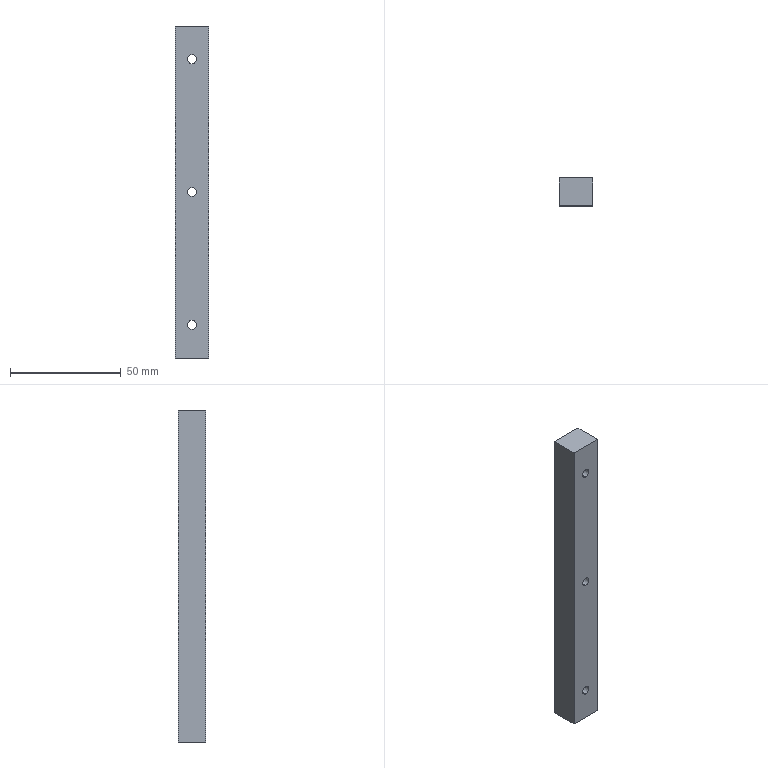Part | SolidWorks | features ICE 3, Extrusion 1, LPattern 1 | 1 solid | 21 faces | box 15 x 12.5 x 150 mm | volume 27442 mm3 | cylinder 12 | plane 9 | commonest cylinder face diameters 4 x6 6 x6
STEP:
#1=CARTESIAN_POINT('',(0.,-6.25,-62.));
#2=VERTEX_POINT('',#1);
#3=CARTESIAN_POINT('',(0.,-6.25,-58.));
#4=VERTEX_POINT('',#3);
#5=CARTESIAN_POINT('',(0.,-6.25,-60.));
#6=DIRECTION('',(0.,1.,0.));
#7=DIRECTION('',(0.,0.,1.));
#8=AXIS2_PLACEMENT_3D('',#5,#6,#7);
#9=CIRCLE('',#8,2.);
#10=EDGE_CURVE('',#2,#4,#9,.T.);
#11=ORIENTED_EDGE('',*,*,#10,.F.);
#12=CARTESIAN_POINT('',(0.,1.75,-62.));
#13=VERTEX_POINT('',#12);
#14=CARTESIAN_POINT('',(0.,-6.25,-62.));
#15=DIRECTION('',(0.,1.,0.));
#16=VECTOR('',#15,1000.);
#17=LINE('',#14,#16);
#18=EDGE_CURVE('',#2,#13,#17,.T.);
#19=ORIENTED_EDGE('',*,*,#18,.T.);
#20=CARTESIAN_POINT('',(0.,1.75,-58.));
#21=VERTEX_POINT('',#20);
#22=CARTESIAN_POINT('',(0.,1.75,-60.));
#23=DIRECTION('',(0.,1.,0.));
#24=DIRECTION('',(0.,0.,1.));
#25=AXIS2_PLACEMENT_3D('',#22,#23,#24);
#26=CIRCLE('',#25,2.);
#27=EDGE_CURVE('',#13,#21,#26,.T.);
#28=ORIENTED_EDGE('',*,*,#27,.T.);
#29=CARTESIAN_POINT('',(0.,-6.25,-58.));
#30=DIRECTION('',(0.,1.,0.));
#31=VECTOR('',#30,1000.);
#32=LINE('',#29,#31);
#33=EDGE_CURVE('',#4,#21,#32,.T.);
#34=ORIENTED_EDGE('',*,*,#33,.F.);
#35=EDGE_LOOP('',(#11,#19,#28,#34));
#36=FACE_OUTER_BOUND('',#35,.T.);
#37=CARTESIAN_POINT('',(0.,-6.25,-60.));
#38=DIRECTION('',(0.,1.,0.));
#39=DIRECTION('',(0.,0.,1.));
#40=AXIS2_PLACEMENT_3D('',#37,#38,#39);
#41=CYLINDRICAL_SURFACE('',#40,2.);
#42=ADVANCED_FACE('',(#36),#41,.F.);
#43=CARTESIAN_POINT('',(0.,-6.25,-2.));
#44=VERTEX_POINT('',#43);
#45=CARTESIAN_POINT('',(0.,-6.25,2.));
#46=VERTEX_POINT('',#45);
#47=CARTESIAN_POINT('',(0.,-6.25,0.));
#48=DIRECTION('',(0.,1.,0.));
#49=DIRECTION('',(0.,0.,1.));
#50=AXIS2_PLACEMENT_3D('',#47,#48,#49);
#51=CIRCLE('',#50,2.);
#52=EDGE_CURVE('',#44,#46,#51,.T.);
#53=ORIENTED_EDGE('',*,*,#52,.F.);
#54=CARTESIAN_POINT('',(0.,1.75,-2.));
#55=VERTEX_POINT('',#54);
#56=CARTESIAN_POINT('',(0.,-6.25,-2.));
#57=DIRECTION('',(0.,1.,0.));
#58=VECTOR('',#57,1000.);
#59=LINE('',#56,#58);
#60=EDGE_CURVE('',#44,#55,#59,.T.);
#61=ORIENTED_EDGE('',*,*,#60,.T.);
#62=CARTESIAN_POINT('',(0.,1.75,2.));
#63=VERTEX_POINT('',#62);
#64=CARTESIAN_POINT('',(0.,1.75,0.));
#65=DIRECTION('',(0.,1.,0.));
#66=DIRECTION('',(0.,0.,1.));
#67=AXIS2_PLACEMENT_3D('',#64,#65,#66);
#68=CIRCLE('',#67,2.);
#69=EDGE_CURVE('',#55,#63,#68,.T.);
#70=ORIENTED_EDGE('',*,*,#69,.T.);
#71=CARTESIAN_POINT('',(0.,-6.25,2.));
#72=DIRECTION('',(0.,1.,0.));
#73=VECTOR('',#72,1000.);
#74=LINE('',#71,#73);
#75=EDGE_CURVE('',#46,#63,#74,.T.);
#76=ORIENTED_EDGE('',*,*,#75,.F.);
#77=EDGE_LOOP('',(#53,#61,#70,#76));
#78=FACE_OUTER_BOUND('',#77,.T.);
#79=CARTESIAN_POINT('',(0.,-6.25,0.));
#80=DIRECTION('',(0.,1.,0.));
#81=DIRECTION('',(0.,0.,1.));
#82=AXIS2_PLACEMENT_3D('',#79,#80,#81);
#83=CYLINDRICAL_SURFACE('',#82,2.);
#84=ADVANCED_FACE('',(#78),#83,.F.);
#85=CARTESIAN_POINT('',(0.,1.75,-63.));
#86=VERTEX_POINT('',#85);
#87=CARTESIAN_POINT('',(0.,1.75,-57.));
#88=VERTEX_POINT('',#87);
#89=CARTESIAN_POINT('',(0.,1.75,-60.));
#90=DIRECTION('',(0.,1.,0.));
#91=DIRECTION('',(0.,0.,1.));
#92=AXIS2_PLACEMENT_3D('',#89,#90,#91);
#93=CIRCLE('',#92,3.);
#94=EDGE_CURVE('',#86,#88,#93,.T.);
#95=ORIENTED_EDGE('',*,*,#94,.F.);
#96=CARTESIAN_POINT('',(0.,6.25,-63.));
#97=VERTEX_POINT('',#96);
#98=CARTESIAN_POINT('',(0.,1.75,-63.));
#99=DIRECTION('',(0.,1.,0.));
#100=VECTOR('',#99,1000.);
#101=LINE('',#98,#100);
#102=EDGE_CURVE('',#86,#97,#101,.T.);
#103=ORIENTED_EDGE('',*,*,#102,.T.);
#104=CARTESIAN_POINT('',(0.,6.25,-57.));
#105=VERTEX_POINT('',#104);
#106=CARTESIAN_POINT('',(0.,6.25,-60.));
#107=DIRECTION('',(0.,1.,0.));
#108=DIRECTION('',(0.,0.,1.));
#109=AXIS2_PLACEMENT_3D('',#106,#107,#108);
#110=CIRCLE('',#109,3.);
#111=EDGE_CURVE('',#97,#105,#110,.T.);
#112=ORIENTED_EDGE('',*,*,#111,.T.);
#113=CARTESIAN_POINT('',(0.,1.75,-57.));
#114=DIRECTION('',(0.,1.,0.));
#115=VECTOR('',#114,1000.);
#116=LINE('',#113,#115);
#117=EDGE_CURVE('',#88,#105,#116,.T.);
#118=ORIENTED_EDGE('',*,*,#117,.F.);
#119=EDGE_LOOP('',(#95,#103,#112,#118));
#120=FACE_OUTER_BOUND('',#119,.T.);
#121=CARTESIAN_POINT('',(0.,1.75,-60.));
#122=DIRECTION('',(0.,1.,0.));
#123=DIRECTION('',(0.,0.,1.));
#124=AXIS2_PLACEMENT_3D('',#121,#122,#123);
#125=CYLINDRICAL_SURFACE('',#124,3.);
#126=ADVANCED_FACE('',(#120),#125,.F.);
#127=CARTESIAN_POINT('',(0.,1.75,-3.));
#128=VERTEX_POINT('',#127);
#129=CARTESIAN_POINT('',(0.,1.75,3.));
#130=VERTEX_POINT('',#129);
#131=CARTESIAN_POINT('',(0.,1.75,0.));
#132=DIRECTION('',(0.,1.,0.));
#133=DIRECTION('',(0.,0.,1.));
#134=AXIS2_PLACEMENT_3D('',#131,#132,#133);
#135=CIRCLE('',#134,3.);
#136=EDGE_CURVE('',#128,#130,#135,.T.);
#137=ORIENTED_EDGE('',*,*,#136,.F.);
#138=CARTESIAN_POINT('',(0.,6.25,-3.));
#139=VERTEX_POINT('',#138);
#140=CARTESIAN_POINT('',(0.,1.75,-3.));
#141=DIRECTION('',(0.,1.,0.));
#142=VECTOR('',#141,1000.);
#143=LINE('',#140,#142);
#144=EDGE_CURVE('',#128,#139,#143,.T.);
#145=ORIENTED_EDGE('',*,*,#144,.T.);
#146=CARTESIAN_POINT('',(0.,6.25,3.));
#147=VERTEX_POINT('',#146);
#148=CARTESIAN_POINT('',(0.,6.25,0.));
#149=DIRECTION('',(0.,1.,0.));
#150=DIRECTION('',(0.,0.,1.));
#151=AXIS2_PLACEMENT_3D('',#148,#149,#150);
#152=CIRCLE('',#151,3.);
#153=EDGE_CURVE('',#139,#147,#152,.T.);
#154=ORIENTED_EDGE('',*,*,#153,.T.);
#155=CARTESIAN_POINT('',(0.,1.75,3.));
#156=DIRECTION('',(0.,1.,0.));
#157=VECTOR('',#156,1000.);
#158=LINE('',#155,#157);
#159=EDGE_CURVE('',#130,#147,#158,.T.);
#160=ORIENTED_EDGE('',*,*,#159,.F.);
#161=EDGE_LOOP('',(#137,#145,#154,#160));
#162=FACE_OUTER_BOUND('',#161,.T.);
#163=CARTESIAN_POINT('',(0.,1.75,0.));
#164=DIRECTION('',(0.,1.,0.));
#165=DIRECTION('',(0.,0.,1.));
#166=AXIS2_PLACEMENT_3D('',#163,#164,#165);
#167=CYLINDRICAL_SURFACE('',#166,3.);
#168=ADVANCED_FACE('',(#162),#167,.F.);
#169=CARTESIAN_POINT('',(0.,-6.25,58.));
#170=VERTEX_POINT('',#169);
#171=CARTESIAN_POINT('',(0.,-6.25,62.));
#172=VERTEX_POINT('',#171);
#173=CARTESIAN_POINT('',(0.,-6.25,60.));
#174=DIRECTION('',(0.,1.,0.));
#175=DIRECTION('',(0.,0.,1.));
#176=AXIS2_PLACEMENT_3D('',#173,#174,#175);
#177=CIRCLE('',#176,2.);
#178=EDGE_CURVE('',#170,#172,#177,.T.);
#179=ORIENTED_EDGE('',*,*,#178,.F.);
#180=CARTESIAN_POINT('',(0.,1.75,58.));
#181=VERTEX_POINT('',#180);
#182=CARTESIAN_POINT('',(0.,-6.25,58.));
#183=DIRECTION('',(0.,1.,0.));
#184=VECTOR('',#183,1000.);
#185=LINE('',#182,#184);
#186=EDGE_CURVE('',#170,#181,#185,.T.);
#187=ORIENTED_EDGE('',*,*,#186,.T.);
#188=CARTESIAN_POINT('',(0.,1.75,62.));
#189=VERTEX_POINT('',#188);
#190=CARTESIAN_POINT('',(0.,1.75,60.));
#191=DIRECTION('',(0.,1.,0.));
#192=DIRECTION('',(0.,0.,1.));
#193=AXIS2_PLACEMENT_3D('',#190,#191,#192);
#194=CIRCLE('',#193,2.);
#195=EDGE_CURVE('',#181,#189,#194,.T.);
#196=ORIENTED_EDGE('',*,*,#195,.T.);
#197=CARTESIAN_POINT('',(0.,-6.25,62.));
#198=DIRECTION('',(0.,1.,0.));
#199=VECTOR('',#198,1000.);
#200=LINE('',#197,#199);
#201=EDGE_CURVE('',#172,#189,#200,.T.);
#202=ORIENTED_EDGE('',*,*,#201,.F.);
#203=EDGE_LOOP('',(#179,#187,#196,#202));
#204=FACE_OUTER_BOUND('',#203,.T.);
#205=CARTESIAN_POINT('',(0.,-6.25,60.));
#206=DIRECTION('',(0.,1.,0.));
#207=DIRECTION('',(0.,0.,1.));
#208=AXIS2_PLACEMENT_3D('',#205,#206,#207);
#209=CYLINDRICAL_SURFACE('',#208,2.);
#210=ADVANCED_FACE('',(#204),#209,.F.);
#211=CARTESIAN_POINT('',(0.,1.75,57.));
#212=VERTEX_POINT('',#211);
#213=CARTESIAN_POINT('',(0.,1.75,63.));
#214=VERTEX_POINT('',#213);
#215=CARTESIAN_POINT('',(0.,1.75,60.));
#216=DIRECTION('',(0.,1.,0.));
#217=DIRECTION('',(0.,0.,1.));
#218=AXIS2_PLACEMENT_3D('',#215,#216,#217);
#219=CIRCLE('',#218,3.);
#220=EDGE_CURVE('',#212,#214,#219,.T.);
#221=ORIENTED_EDGE('',*,*,#220,.F.);
#222=CARTESIAN_POINT('',(0.,6.25,57.));
#223=VERTEX_POINT('',#222);
#224=CARTESIAN_POINT('',(0.,1.75,57.));
#225=DIRECTION('',(0.,1.,0.));
#226=VECTOR('',#225,1000.);
#227=LINE('',#224,#226);
#228=EDGE_CURVE('',#212,#223,#227,.T.);
#229=ORIENTED_EDGE('',*,*,#228,.T.);
#230=CARTESIAN_POINT('',(0.,6.25,63.));
#231=VERTEX_POINT('',#230);
#232=CARTESIAN_POINT('',(0.,6.25,60.));
#233=DIRECTION('',(0.,1.,0.));
#234=DIRECTION('',(0.,0.,1.));
#235=AXIS2_PLACEMENT_3D('',#232,#233,#234);
#236=CIRCLE('',#235,3.);
#237=EDGE_CURVE('',#223,#231,#236,.T.);
#238=ORIENTED_EDGE('',*,*,#237,.T.);
#239=CARTESIAN_POINT('',(0.,1.75,63.));
#240=DIRECTION('',(0.,1.,0.));
#241=VECTOR('',#240,1000.);
#242=LINE('',#239,#241);
#243=EDGE_CURVE('',#214,#231,#242,.T.);
#244=ORIENTED_EDGE('',*,*,#243,.F.);
#245=EDGE_LOOP('',(#221,#229,#238,#244));
#246=FACE_OUTER_BOUND('',#245,.T.);
#247=CARTESIAN_POINT('',(0.,1.75,60.));
#248=DIRECTION('',(0.,1.,0.));
#249=DIRECTION('',(0.,0.,1.));
#250=AXIS2_PLACEMENT_3D('',#247,#248,#249);
#251=CYLINDRICAL_SURFACE('',#250,3.);
#252=ADVANCED_FACE('',(#246),#251,.F.);
#253=CARTESIAN_POINT('',(7.5,-6.25,-75.));
#254=VERTEX_POINT('',#253);
#255=CARTESIAN_POINT('',(7.5,6.25,-75.));
#256=VERTEX_POINT('',#255);
#257=CARTESIAN_POINT('',(7.5,6.25,-75.));
#258=DIRECTION('',(0.,1.,0.));
#259=VECTOR('',#258,1000.);
#260=LINE('',#257,#259);
#261=EDGE_CURVE('',#254,#256,#260,.T.);
#262=ORIENTED_EDGE('',*,*,#261,.T.);
#263=CARTESIAN_POINT('',(7.5,6.25,75.));
#264=VERTEX_POINT('',#263);
#265=CARTESIAN_POINT('',(7.5,6.25,75.));
#266=DIRECTION('',(0.,0.,-1.));
#267=VECTOR('',#266,1000.);
#268=LINE('',#265,#267);
#269=EDGE_CURVE('',#264,#256,#268,.T.);
#270=ORIENTED_EDGE('',*,*,#269,.F.);
#271=CARTESIAN_POINT('',(7.5,-6.25,75.));
#272=VERTEX_POINT('',#271);
#273=CARTESIAN_POINT('',(7.5,6.25,75.));
#274=DIRECTION('',(0.,1.,0.));
#275=VECTOR('',#274,1000.);
#276=LINE('',#273,#275);
#277=EDGE_CURVE('',#272,#264,#276,.T.);
#278=ORIENTED_EDGE('',*,*,#277,.F.);
#279=CARTESIAN_POINT('',(7.5,-6.25,75.));
#280=DIRECTION('',(0.,0.,-1.));
#281=VECTOR('',#280,1000.);
#282=LINE('',#279,#281);
#283=EDGE_CURVE('',#272,#254,#282,.T.);
#284=ORIENTED_EDGE('',*,*,#283,.T.);
#285=EDGE_LOOP('',(#262,#270,#278,#284));
#286=FACE_OUTER_BOUND('',#285,.T.);
#287=CARTESIAN_POINT('',(7.5,6.25,75.));
#288=DIRECTION('',(-1.,0.,0.));
#289=DIRECTION('',(0.,-1.,0.));
#290=AXIS2_PLACEMENT_3D('',#287,#288,#289);
#291=PLANE('',#290);
#292=ADVANCED_FACE('',(#286),#291,.F.);
#293=CARTESIAN_POINT('',(0.,6.25,-60.));
#294=DIRECTION('',(0.,1.,0.));
#295=DIRECTION('',(0.,0.,1.));
#296=AXIS2_PLACEMENT_3D('',#293,#294,#295);
#297=CIRCLE('',#296,3.);
#298=EDGE_CURVE('',#105,#97,#297,.T.);
#299=ORIENTED_EDGE('',*,*,#298,.F.);
#300=ORIENTED_EDGE('',*,*,#111,.F.);
#301=EDGE_LOOP('',(#299,#300));
#302=FACE_BOUND('',#301,.T.);
#303=CARTESIAN_POINT('',(0.,6.25,0.));
#304=DIRECTION('',(0.,1.,0.));
#305=DIRECTION('',(0.,0.,1.));
#306=AXIS2_PLACEMENT_3D('',#303,#304,#305);
#307=CIRCLE('',#306,3.);
#308=EDGE_CURVE('',#147,#139,#307,.T.);
#309=ORIENTED_EDGE('',*,*,#308,.F.);
#310=ORIENTED_EDGE('',*,*,#153,.F.);
#311=EDGE_LOOP('',(#309,#310));
#312=FACE_BOUND('',#311,.T.);
#313=CARTESIAN_POINT('',(0.,6.25,60.));
#314=DIRECTION('',(0.,1.,0.));
#315=DIRECTION('',(0.,0.,1.));
#316=AXIS2_PLACEMENT_3D('',#313,#314,#315);
#317=CIRCLE('',#316,3.);
#318=EDGE_CURVE('',#231,#223,#317,.T.);
#319=ORIENTED_EDGE('',*,*,#318,.F.);
#320=ORIENTED_EDGE('',*,*,#237,.F.);
#321=EDGE_LOOP('',(#319,#320));
#322=FACE_BOUND('',#321,.T.);
#323=CARTESIAN_POINT('',(-7.5,6.25,-75.));
#324=VERTEX_POINT('',#323);
#325=CARTESIAN_POINT('',(-7.5,6.25,-75.));
#326=DIRECTION('',(-1.,0.,0.));
#327=VECTOR('',#326,1000.);
#328=LINE('',#325,#327);
#329=EDGE_CURVE('',#256,#324,#328,.T.);
#330=ORIENTED_EDGE('',*,*,#329,.T.);
#331=CARTESIAN_POINT('',(-7.5,6.25,75.));
#332=VERTEX_POINT('',#331);
#333=CARTESIAN_POINT('',(-7.5,6.25,75.));
#334=DIRECTION('',(0.,0.,-1.));
#335=VECTOR('',#334,1000.);
#336=LINE('',#333,#335);
#337=EDGE_CURVE('',#332,#324,#336,.T.);
#338=ORIENTED_EDGE('',*,*,#337,.F.);
#339=CARTESIAN_POINT('',(-7.5,6.25,75.));
#340=DIRECTION('',(-1.,0.,0.));
#341=VECTOR('',#340,1000.);
#342=LINE('',#339,#341);
#343=EDGE_CURVE('',#264,#332,#342,.T.);
#344=ORIENTED_EDGE('',*,*,#343,.F.);
#345=ORIENTED_EDGE('',*,*,#269,.T.);
#346=EDGE_LOOP('',(#330,#338,#344,#345));
#347=FACE_OUTER_BOUND('',#346,.T.);
#348=CARTESIAN_POINT('',(-7.5,6.25,75.));
#349=DIRECTION('',(0.,-1.,0.));
#350=DIRECTION('',(0.,0.,-1.));
#351=AXIS2_PLACEMENT_3D('',#348,#349,#350);
#352=PLANE('',#351);
#353=ADVANCED_FACE('',(#302,#312,#322,#347),#352,.F.);
#354=CARTESIAN_POINT('',(-7.5,-6.25,-75.));
#355=VERTEX_POINT('',#354);
#356=CARTESIAN_POINT('',(-7.5,6.25,-75.));
#357=DIRECTION('',(0.,-1.,0.));
#358=VECTOR('',#357,1000.);
#359=LINE('',#356,#358);
#360=EDGE_CURVE('',#324,#355,#359,.T.);
#361=ORIENTED_EDGE('',*,*,#360,.T.);
#362=CARTESIAN_POINT('',(-7.5,-6.25,75.));
#363=VERTEX_POINT('',#362);
#364=CARTESIAN_POINT('',(-7.5,-6.25,75.));
#365=DIRECTION('',(0.,0.,-1.));
#366=VECTOR('',#365,1000.);
#367=LINE('',#364,#366);
#368=EDGE_CURVE('',#363,#355,#367,.T.);
#369=ORIENTED_EDGE('',*,*,#368,.F.);
#370=CARTESIAN_POINT('',(-7.5,6.25,75.));
#371=DIRECTION('',(0.,-1.,0.));
#372=VECTOR('',#371,1000.);
#373=LINE('',#370,#372);
#374=EDGE_CURVE('',#332,#363,#373,.T.);
#375=ORIENTED_EDGE('',*,*,#374,.F.);
#376=ORIENTED_EDGE('',*,*,#337,.T.);
#377=EDGE_LOOP('',(#361,#369,#375,#376));
#378=FACE_OUTER_BOUND('',#377,.T.);
#379=CARTESIAN_POINT('',(-7.5,6.25,75.));
#380=DIRECTION('',(1.,0.,0.));
#381=DIRECTION('',(0.,1.,0.));
#382=AXIS2_PLACEMENT_3D('',#379,#380,#381);
#383=PLANE('',#382);
#384=ADVANCED_FACE('',(#378),#383,.F.);
#385=CARTESIAN_POINT('',(0.,-6.25,-60.));
#386=DIRECTION('',(0.,1.,0.));
#387=DIRECTION('',(0.,0.,1.));
#388=AXIS2_PLACEMENT_3D('',#385,#386,#387);
#389=CIRCLE('',#388,2.);
#390=EDGE_CURVE('',#4,#2,#389,.T.);
#391=ORIENTED_EDGE('',*,*,#390,.T.);
#392=ORIENTED_EDGE('',*,*,#10,.T.);
#393=EDGE_LOOP('',(#391,#392));
#394=FACE_BOUND('',#393,.T.);
#395=CARTESIAN_POINT('',(0.,-6.25,0.));
#396=DIRECTION('',(0.,1.,0.));
#397=DIRECTION('',(0.,0.,1.));
#398=AXIS2_PLACEMENT_3D('',#395,#396,#397);
#399=CIRCLE('',#398,2.);
#400=EDGE_CURVE('',#46,#44,#399,.T.);
#401=ORIENTED_EDGE('',*,*,#400,.T.);
#402=ORIENTED_EDGE('',*,*,#52,.T.);
#403=EDGE_LOOP('',(#401,#402));
#404=FACE_BOUND('',#403,.T.);
#405=CARTESIAN_POINT('',(0.,-6.25,60.));
#406=DIRECTION('',(0.,1.,0.));
#407=DIRECTION('',(0.,0.,1.));
#408=AXIS2_PLACEMENT_3D('',#405,#406,#407);
#409=CIRCLE('',#408,2.);
#410=EDGE_CURVE('',#172,#170,#409,.T.);
#411=ORIENTED_EDGE('',*,*,#410,.T.);
#412=ORIENTED_EDGE('',*,*,#178,.T.);
#413=EDGE_LOOP('',(#411,#412));
#414=FACE_BOUND('',#413,.T.);
#415=CARTESIAN_POINT('',(-7.5,-6.25,-75.));
#416=DIRECTION('',(1.,0.,0.));
#417=VECTOR('',#416,1000.);
#418=LINE('',#415,#417);
#419=EDGE_CURVE('',#355,#254,#418,.T.);
#420=ORIENTED_EDGE('',*,*,#419,.T.);
#421=ORIENTED_EDGE('',*,*,#283,.F.);
#422=CARTESIAN_POINT('',(-7.5,-6.25,75.));
#423=DIRECTION('',(1.,0.,0.));
#424=VECTOR('',#423,1000.);
#425=LINE('',#422,#424);
#426=EDGE_CURVE('',#363,#272,#425,.T.);
#427=ORIENTED_EDGE('',*,*,#426,.F.);
#428=ORIENTED_EDGE('',*,*,#368,.T.);
#429=EDGE_LOOP('',(#420,#421,#427,#428));
#430=FACE_OUTER_BOUND('',#429,.T.);
#431=CARTESIAN_POINT('',(-7.5,-6.25,75.));
#432=DIRECTION('',(0.,1.,0.));
#433=DIRECTION('',(0.,0.,1.));
#434=AXIS2_PLACEMENT_3D('',#431,#432,#433);
#435=PLANE('',#434);
#436=ADVANCED_FACE('',(#394,#404,#414,#430),#435,.F.);
#437=ORIENTED_EDGE('',*,*,#277,.T.);
#438=ORIENTED_EDGE('',*,*,#343,.T.);
#439=ORIENTED_EDGE('',*,*,#374,.T.);
#440=ORIENTED_EDGE('',*,*,#426,.T.);
#441=EDGE_LOOP('',(#437,#438,#439,#440));
#442=FACE_OUTER_BOUND('',#441,.T.);
#443=CARTESIAN_POINT('',(0.,0.,75.));
#444=DIRECTION('',(0.,0.,1.));
#445=DIRECTION('',(1.,0.,0.));
#446=AXIS2_PLACEMENT_3D('',#443,#444,#445);
#447=PLANE('',#446);
#448=ADVANCED_FACE('',(#442),#447,.T.);
#449=ORIENTED_EDGE('',*,*,#261,.F.);
#450=ORIENTED_EDGE('',*,*,#419,.F.);
#451=ORIENTED_EDGE('',*,*,#360,.F.);
#452=ORIENTED_EDGE('',*,*,#329,.F.);
#453=EDGE_LOOP('',(#449,#450,#451,#452));
#454=FACE_OUTER_BOUND('',#453,.T.);
#455=CARTESIAN_POINT('',(0.,0.,-75.));
#456=DIRECTION('',(0.,0.,1.));
#457=DIRECTION('',(1.,0.,0.));
#458=AXIS2_PLACEMENT_3D('',#455,#456,#457);
#459=PLANE('',#458);
#460=ADVANCED_FACE('',(#454),#459,.F.);
#461=ORIENTED_EDGE('',*,*,#228,.F.);
#462=CARTESIAN_POINT('',(0.,1.75,60.));
#463=DIRECTION('',(0.,1.,0.));
#464=DIRECTION('',(0.,0.,1.));
#465=AXIS2_PLACEMENT_3D('',#462,#463,#464);
#466=CIRCLE('',#465,3.);
#467=EDGE_CURVE('',#214,#212,#466,.T.);
#468=ORIENTED_EDGE('',*,*,#467,.F.);
#469=ORIENTED_EDGE('',*,*,#243,.T.);
#470=ORIENTED_EDGE('',*,*,#318,.T.);
#471=EDGE_LOOP('',(#461,#468,#469,#470));
#472=FACE_OUTER_BOUND('',#471,.T.);
#473=CARTESIAN_POINT('',(0.,1.75,60.));
#474=DIRECTION('',(0.,1.,0.));
#475=DIRECTION('',(0.,0.,1.));
#476=AXIS2_PLACEMENT_3D('',#473,#474,#475);
#477=CYLINDRICAL_SURFACE('',#476,3.);
#478=ADVANCED_FACE('',(#472),#477,.F.);
#479=CARTESIAN_POINT('',(0.,1.75,60.));
#480=DIRECTION('',(0.,1.,0.));
#481=DIRECTION('',(0.,0.,1.));
#482=AXIS2_PLACEMENT_3D('',#479,#480,#481);
#483=CIRCLE('',#482,2.);
#484=EDGE_CURVE('',#189,#181,#483,.T.);
#485=ORIENTED_EDGE('',*,*,#484,.F.);
#486=ORIENTED_EDGE('',*,*,#195,.F.);
#487=EDGE_LOOP('',(#485,#486));
#488=FACE_BOUND('',#487,.T.);
#489=ORIENTED_EDGE('',*,*,#467,.T.);
#490=ORIENTED_EDGE('',*,*,#220,.T.);
#491=EDGE_LOOP('',(#489,#490));
#492=FACE_OUTER_BOUND('',#491,.T.);
#493=CARTESIAN_POINT('',(0.,1.75,60.));
#494=DIRECTION('',(0.,1.,0.));
#495=DIRECTION('',(0.,0.,1.));
#496=AXIS2_PLACEMENT_3D('',#493,#494,#495);
#497=PLANE('',#496);
#498=ADVANCED_FACE('',(#488,#492),#497,.T.);
#499=ORIENTED_EDGE('',*,*,#186,.F.);
#500=ORIENTED_EDGE('',*,*,#410,.F.);
#501=ORIENTED_EDGE('',*,*,#201,.T.);
#502=ORIENTED_EDGE('',*,*,#484,.T.);
#503=EDGE_LOOP('',(#499,#500,#501,#502));
#504=FACE_OUTER_BOUND('',#503,.T.);
#505=CARTESIAN_POINT('',(0.,-6.25,60.));
#506=DIRECTION('',(0.,1.,0.));
#507=DIRECTION('',(0.,0.,1.));
#508=AXIS2_PLACEMENT_3D('',#505,#506,#507);
#509=CYLINDRICAL_SURFACE('',#508,2.);
#510=ADVANCED_FACE('',(#504),#509,.F.);
#511=ORIENTED_EDGE('',*,*,#144,.F.);
#512=CARTESIAN_POINT('',(0.,1.75,0.));
#513=DIRECTION('',(0.,1.,0.));
#514=DIRECTION('',(0.,0.,1.));
#515=AXIS2_PLACEMENT_3D('',#512,#513,#514);
#516=CIRCLE('',#515,3.);
#517=EDGE_CURVE('',#130,#128,#516,.T.);
#518=ORIENTED_EDGE('',*,*,#517,.F.);
#519=ORIENTED_EDGE('',*,*,#159,.T.);
#520=ORIENTED_EDGE('',*,*,#308,.T.);
#521=EDGE_LOOP('',(#511,#518,#519,#520));
#522=FACE_OUTER_BOUND('',#521,.T.);
#523=CARTESIAN_POINT('',(0.,1.75,0.));
#524=DIRECTION('',(0.,1.,0.));
#525=DIRECTION('',(0.,0.,1.));
#526=AXIS2_PLACEMENT_3D('',#523,#524,#525);
#527=CYLINDRICAL_SURFACE('',#526,3.);
#528=ADVANCED_FACE('',(#522),#527,.F.);
#529=CARTESIAN_POINT('',(0.,1.75,0.));
#530=DIRECTION('',(0.,1.,0.));
#531=DIRECTION('',(0.,0.,1.));
#532=AXIS2_PLACEMENT_3D('',#529,#530,#531);
#533=CIRCLE('',#532,2.);
#534=EDGE_CURVE('',#63,#55,#533,.T.);
#535=ORIENTED_EDGE('',*,*,#534,.F.);
#536=ORIENTED_EDGE('',*,*,#69,.F.);
#537=EDGE_LOOP('',(#535,#536));
#538=FACE_BOUND('',#537,.T.);
#539=ORIENTED_EDGE('',*,*,#517,.T.);
#540=ORIENTED_EDGE('',*,*,#136,.T.);
#541=EDGE_LOOP('',(#539,#540));
#542=FACE_OUTER_BOUND('',#541,.T.);
#543=CARTESIAN_POINT('',(0.,1.75,0.));
#544=DIRECTION('',(0.,1.,0.));
#545=DIRECTION('',(0.,0.,1.));
#546=AXIS2_PLACEMENT_3D('',#543,#544,#545);
#547=PLANE('',#546);
#548=ADVANCED_FACE('',(#538,#542),#547,.T.);
#549=ORIENTED_EDGE('',*,*,#102,.F.);
#550=CARTESIAN_POINT('',(0.,1.75,-60.));
#551=DIRECTION('',(0.,1.,0.));
#552=DIRECTION('',(0.,0.,1.));
#553=AXIS2_PLACEMENT_3D('',#550,#551,#552);
#554=CIRCLE('',#553,3.);
#555=EDGE_CURVE('',#88,#86,#554,.T.);
#556=ORIENTED_EDGE('',*,*,#555,.F.);
#557=ORIENTED_EDGE('',*,*,#117,.T.);
#558=ORIENTED_EDGE('',*,*,#298,.T.);
#559=EDGE_LOOP('',(#549,#556,#557,#558));
#560=FACE_OUTER_BOUND('',#559,.T.);
#561=CARTESIAN_POINT('',(0.,1.75,-60.));
#562=DIRECTION('',(0.,1.,0.));
#563=DIRECTION('',(0.,0.,1.));
#564=AXIS2_PLACEMENT_3D('',#561,#562,#563);
#565=CYLINDRICAL_SURFACE('',#564,3.);
#566=ADVANCED_FACE('',(#560),#565,.F.);
#567=CARTESIAN_POINT('',(0.,1.75,-60.));
#568=DIRECTION('',(0.,1.,0.));
#569=DIRECTION('',(0.,0.,1.));
#570=AXIS2_PLACEMENT_3D('',#567,#568,#569);
#571=CIRCLE('',#570,2.);
#572=EDGE_CURVE('',#21,#13,#571,.T.);
#573=ORIENTED_EDGE('',*,*,#572,.F.);
#574=ORIENTED_EDGE('',*,*,#27,.F.);
#575=EDGE_LOOP('',(#573,#574));
#576=FACE_BOUND('',#575,.T.);
#577=ORIENTED_EDGE('',*,*,#555,.T.);
#578=ORIENTED_EDGE('',*,*,#94,.T.);
#579=EDGE_LOOP('',(#577,#578));
#580=FACE_OUTER_BOUND('',#579,.T.);
#581=CARTESIAN_POINT('',(0.,1.75,-60.));
#582=DIRECTION('',(0.,1.,0.));
#583=DIRECTION('',(0.,0.,1.));
#584=AXIS2_PLACEMENT_3D('',#581,#582,#583);
#585=PLANE('',#584);
#586=ADVANCED_FACE('',(#576,#580),#585,.T.);
#587=ORIENTED_EDGE('',*,*,#60,.F.);
#588=ORIENTED_EDGE('',*,*,#400,.F.);
#589=ORIENTED_EDGE('',*,*,#75,.T.);
#590=ORIENTED_EDGE('',*,*,#534,.T.);
#591=EDGE_LOOP('',(#587,#588,#589,#590));
#592=FACE_OUTER_BOUND('',#591,.T.);
#593=CARTESIAN_POINT('',(0.,-6.25,0.));
#594=DIRECTION('',(0.,1.,0.));
#595=DIRECTION('',(0.,0.,1.));
#596=AXIS2_PLACEMENT_3D('',#593,#594,#595);
#597=CYLINDRICAL_SURFACE('',#596,2.);
#598=ADVANCED_FACE('',(#592),#597,.F.);
#599=ORIENTED_EDGE('',*,*,#18,.F.);
#600=ORIENTED_EDGE('',*,*,#390,.F.);
#601=ORIENTED_EDGE('',*,*,#33,.T.);
#602=ORIENTED_EDGE('',*,*,#572,.T.);
#603=EDGE_LOOP('',(#599,#600,#601,#602));
#604=FACE_OUTER_BOUND('',#603,.T.);
#605=CARTESIAN_POINT('',(0.,-6.25,-60.));
#606=DIRECTION('',(0.,1.,0.));
#607=DIRECTION('',(0.,0.,1.));
#608=AXIS2_PLACEMENT_3D('',#605,#606,#607);
#609=CYLINDRICAL_SURFACE('',#608,2.);
#610=ADVANCED_FACE('',(#604),#609,.F.);
#611=CLOSED_SHELL('',(#42,#84,#126,#168,#210,#252,#292,#353,#384,#436,#448,#460,#478,#498,#510,#528,#548,#566,#586,#598,#610));
#612=MANIFOLD_SOLID_BREP('',#611);
#613=CARTESIAN_POINT('',(0.,0.,0.));
#614=DIRECTION('',(0.,0.,1.));
#615=DIRECTION('',(1.,0.,0.));
#616=AXIS2_PLACEMENT_3D('',#613,#614,#615);
#617=(LENGTH_UNIT()NAMED_UNIT(*)SI_UNIT(.MILLI.,.METRE.));
#618=UNCERTAINTY_MEASURE_WITH_UNIT(LENGTH_MEASURE(0.00001),#617,'','');
#619=(NAMED_UNIT(*)PLANE_ANGLE_UNIT()SI_UNIT($,.RADIAN.));
#620=(NAMED_UNIT(*)SI_UNIT($,.STERADIAN.)SOLID_ANGLE_UNIT());
#621=(GEOMETRIC_REPRESENTATION_CONTEXT(3)GLOBAL_UNCERTAINTY_ASSIGNED_CONTEXT((#618))GLOBAL_UNIT_ASSIGNED_CONTEXT((#617,#619,#620))REPRESENTATION_CONTEXT('',''));
#622=ADVANCED_BREP_SHAPE_REPRESENTATION('',(#612,#616),#621);